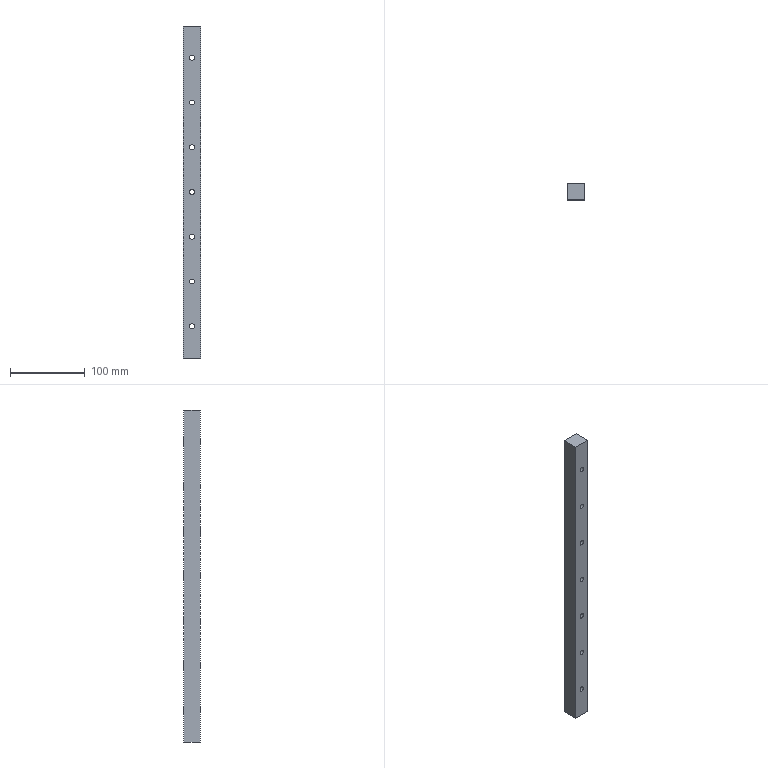Part | SolidWorks | features Extrusion 1, HoleWzd 1, LPattern 1 | 1 solid | 41 faces | box 23 x 22 x 445 mm | volume 217006 mm3 | cylinder 28 | plane 13 | commonest cylinder face diameters 6.6 x14 11 x14
STEP:
#1=CARTESIAN_POINT('',(0.,15.2,37.));
#2=VERTEX_POINT('',#1);
#3=CARTESIAN_POINT('',(0.,15.2,48.));
#4=VERTEX_POINT('',#3);
#5=CARTESIAN_POINT('',(0.,15.2,42.5));
#6=DIRECTION('',(0.,1.,0.));
#7=DIRECTION('',(0.,0.,1.));
#8=AXIS2_PLACEMENT_3D('',#5,#6,#7);
#9=CIRCLE('',#8,5.5);
#10=EDGE_CURVE('',#2,#4,#9,.T.);
#11=ORIENTED_EDGE('',*,*,#10,.F.);
#12=CARTESIAN_POINT('',(0.,22.,37.));
#13=VERTEX_POINT('',#12);
#14=CARTESIAN_POINT('',(0.,22.,37.));
#15=DIRECTION('',(0.,1.,0.));
#16=VECTOR('',#15,1000.);
#17=LINE('',#14,#16);
#18=EDGE_CURVE('',#2,#13,#17,.T.);
#19=ORIENTED_EDGE('',*,*,#18,.T.);
#20=CARTESIAN_POINT('',(0.,22.,48.));
#21=VERTEX_POINT('',#20);
#22=CARTESIAN_POINT('',(0.,22.,42.5));
#23=DIRECTION('',(0.,1.,0.));
#24=DIRECTION('',(0.,0.,1.));
#25=AXIS2_PLACEMENT_3D('',#22,#23,#24);
#26=CIRCLE('',#25,5.5);
#27=EDGE_CURVE('',#13,#21,#26,.T.);
#28=ORIENTED_EDGE('',*,*,#27,.T.);
#29=CARTESIAN_POINT('',(0.,22.,48.));
#30=DIRECTION('',(0.,1.,0.));
#31=VECTOR('',#30,1000.);
#32=LINE('',#29,#31);
#33=EDGE_CURVE('',#4,#21,#32,.T.);
#34=ORIENTED_EDGE('',*,*,#33,.F.);
#35=EDGE_LOOP('',(#11,#19,#28,#34));
#36=FACE_OUTER_BOUND('',#35,.T.);
#37=CARTESIAN_POINT('',(0.,22.,42.5));
#38=DIRECTION('',(0.,1.,0.));
#39=DIRECTION('',(0.,0.,1.));
#40=AXIS2_PLACEMENT_3D('',#37,#38,#39);
#41=CYLINDRICAL_SURFACE('',#40,5.5);
#42=ADVANCED_FACE('',(#36),#41,.F.);
#43=CARTESIAN_POINT('',(0.,0.,39.2));
#44=VERTEX_POINT('',#43);
#45=CARTESIAN_POINT('',(0.,0.,45.8));
#46=VERTEX_POINT('',#45);
#47=CARTESIAN_POINT('',(0.,0.,42.5));
#48=DIRECTION('',(0.,1.,0.));
#49=DIRECTION('',(0.,0.,1.));
#50=AXIS2_PLACEMENT_3D('',#47,#48,#49);
#51=CIRCLE('',#50,3.3);
#52=EDGE_CURVE('',#44,#46,#51,.T.);
#53=ORIENTED_EDGE('',*,*,#52,.F.);
#54=CARTESIAN_POINT('',(0.,15.2,39.2));
#55=VERTEX_POINT('',#54);
#56=CARTESIAN_POINT('',(0.,22.,39.2));
#57=DIRECTION('',(0.,1.,0.));
#58=VECTOR('',#57,1000.);
#59=LINE('',#56,#58);
#60=EDGE_CURVE('',#44,#55,#59,.T.);
#61=ORIENTED_EDGE('',*,*,#60,.T.);
#62=CARTESIAN_POINT('',(0.,15.2,45.8));
#63=VERTEX_POINT('',#62);
#64=CARTESIAN_POINT('',(0.,15.2,42.5));
#65=DIRECTION('',(0.,1.,0.));
#66=DIRECTION('',(0.,0.,1.));
#67=AXIS2_PLACEMENT_3D('',#64,#65,#66);
#68=CIRCLE('',#67,3.3);
#69=EDGE_CURVE('',#55,#63,#68,.T.);
#70=ORIENTED_EDGE('',*,*,#69,.T.);
#71=CARTESIAN_POINT('',(0.,22.,45.8));
#72=DIRECTION('',(0.,1.,0.));
#73=VECTOR('',#72,1000.);
#74=LINE('',#71,#73);
#75=EDGE_CURVE('',#46,#63,#74,.T.);
#76=ORIENTED_EDGE('',*,*,#75,.F.);
#77=EDGE_LOOP('',(#53,#61,#70,#76));
#78=FACE_OUTER_BOUND('',#77,.T.);
#79=CARTESIAN_POINT('',(0.,22.,42.5));
#80=DIRECTION('',(0.,1.,0.));
#81=DIRECTION('',(0.,0.,1.));
#82=AXIS2_PLACEMENT_3D('',#79,#80,#81);
#83=CYLINDRICAL_SURFACE('',#82,3.3);
#84=ADVANCED_FACE('',(#78),#83,.F.);
#85=CARTESIAN_POINT('',(0.,15.2,97.));
#86=VERTEX_POINT('',#85);
#87=CARTESIAN_POINT('',(0.,15.2,108.));
#88=VERTEX_POINT('',#87);
#89=CARTESIAN_POINT('',(0.,15.2,102.5));
#90=DIRECTION('',(0.,1.,0.));
#91=DIRECTION('',(0.,0.,1.));
#92=AXIS2_PLACEMENT_3D('',#89,#90,#91);
#93=CIRCLE('',#92,5.5);
#94=EDGE_CURVE('',#86,#88,#93,.T.);
#95=ORIENTED_EDGE('',*,*,#94,.F.);
#96=CARTESIAN_POINT('',(0.,22.,97.));
#97=VERTEX_POINT('',#96);
#98=CARTESIAN_POINT('',(0.,22.,97.));
#99=DIRECTION('',(0.,1.,0.));
#100=VECTOR('',#99,1000.);
#101=LINE('',#98,#100);
#102=EDGE_CURVE('',#86,#97,#101,.T.);
#103=ORIENTED_EDGE('',*,*,#102,.T.);
#104=CARTESIAN_POINT('',(0.,22.,108.));
#105=VERTEX_POINT('',#104);
#106=CARTESIAN_POINT('',(0.,22.,102.5));
#107=DIRECTION('',(0.,1.,0.));
#108=DIRECTION('',(0.,0.,1.));
#109=AXIS2_PLACEMENT_3D('',#106,#107,#108);
#110=CIRCLE('',#109,5.5);
#111=EDGE_CURVE('',#97,#105,#110,.T.);
#112=ORIENTED_EDGE('',*,*,#111,.T.);
#113=CARTESIAN_POINT('',(0.,22.,108.));
#114=DIRECTION('',(0.,1.,0.));
#115=VECTOR('',#114,1000.);
#116=LINE('',#113,#115);
#117=EDGE_CURVE('',#88,#105,#116,.T.);
#118=ORIENTED_EDGE('',*,*,#117,.F.);
#119=EDGE_LOOP('',(#95,#103,#112,#118));
#120=FACE_OUTER_BOUND('',#119,.T.);
#121=CARTESIAN_POINT('',(0.,22.,102.5));
#122=DIRECTION('',(0.,1.,0.));
#123=DIRECTION('',(0.,0.,1.));
#124=AXIS2_PLACEMENT_3D('',#121,#122,#123);
#125=CYLINDRICAL_SURFACE('',#124,5.5);
#126=ADVANCED_FACE('',(#120),#125,.F.);
#127=CARTESIAN_POINT('',(0.,0.,99.2));
#128=VERTEX_POINT('',#127);
#129=CARTESIAN_POINT('',(0.,0.,105.8));
#130=VERTEX_POINT('',#129);
#131=CARTESIAN_POINT('',(0.,0.,102.5));
#132=DIRECTION('',(0.,1.,0.));
#133=DIRECTION('',(0.,0.,1.));
#134=AXIS2_PLACEMENT_3D('',#131,#132,#133);
#135=CIRCLE('',#134,3.3);
#136=EDGE_CURVE('',#128,#130,#135,.T.);
#137=ORIENTED_EDGE('',*,*,#136,.F.);
#138=CARTESIAN_POINT('',(0.,15.2,99.2));
#139=VERTEX_POINT('',#138);
#140=CARTESIAN_POINT('',(0.,22.,99.2));
#141=DIRECTION('',(0.,1.,0.));
#142=VECTOR('',#141,1000.);
#143=LINE('',#140,#142);
#144=EDGE_CURVE('',#128,#139,#143,.T.);
#145=ORIENTED_EDGE('',*,*,#144,.T.);
#146=CARTESIAN_POINT('',(0.,15.2,105.8));
#147=VERTEX_POINT('',#146);
#148=CARTESIAN_POINT('',(0.,15.2,102.5));
#149=DIRECTION('',(0.,1.,0.));
#150=DIRECTION('',(0.,0.,1.));
#151=AXIS2_PLACEMENT_3D('',#148,#149,#150);
#152=CIRCLE('',#151,3.3);
#153=EDGE_CURVE('',#139,#147,#152,.T.);
#154=ORIENTED_EDGE('',*,*,#153,.T.);
#155=CARTESIAN_POINT('',(0.,22.,105.8));
#156=DIRECTION('',(0.,1.,0.));
#157=VECTOR('',#156,1000.);
#158=LINE('',#155,#157);
#159=EDGE_CURVE('',#130,#147,#158,.T.);
#160=ORIENTED_EDGE('',*,*,#159,.F.);
#161=EDGE_LOOP('',(#137,#145,#154,#160));
#162=FACE_OUTER_BOUND('',#161,.T.);
#163=CARTESIAN_POINT('',(0.,22.,102.5));
#164=DIRECTION('',(0.,1.,0.));
#165=DIRECTION('',(0.,0.,1.));
#166=AXIS2_PLACEMENT_3D('',#163,#164,#165);
#167=CYLINDRICAL_SURFACE('',#166,3.3);
#168=ADVANCED_FACE('',(#162),#167,.F.);
#169=CARTESIAN_POINT('',(0.,15.2,157.));
#170=VERTEX_POINT('',#169);
#171=CARTESIAN_POINT('',(0.,15.2,168.));
#172=VERTEX_POINT('',#171);
#173=CARTESIAN_POINT('',(0.,15.2,162.5));
#174=DIRECTION('',(0.,1.,0.));
#175=DIRECTION('',(0.,0.,1.));
#176=AXIS2_PLACEMENT_3D('',#173,#174,#175);
#177=CIRCLE('',#176,5.5);
#178=EDGE_CURVE('',#170,#172,#177,.T.);
#179=ORIENTED_EDGE('',*,*,#178,.F.);
#180=CARTESIAN_POINT('',(0.,22.,157.));
#181=VERTEX_POINT('',#180);
#182=CARTESIAN_POINT('',(0.,22.,157.));
#183=DIRECTION('',(0.,1.,0.));
#184=VECTOR('',#183,1000.);
#185=LINE('',#182,#184);
#186=EDGE_CURVE('',#170,#181,#185,.T.);
#187=ORIENTED_EDGE('',*,*,#186,.T.);
#188=CARTESIAN_POINT('',(0.,22.,168.));
#189=VERTEX_POINT('',#188);
#190=CARTESIAN_POINT('',(0.,22.,162.5));
#191=DIRECTION('',(0.,1.,0.));
#192=DIRECTION('',(0.,0.,1.));
#193=AXIS2_PLACEMENT_3D('',#190,#191,#192);
#194=CIRCLE('',#193,5.5);
#195=EDGE_CURVE('',#181,#189,#194,.T.);
#196=ORIENTED_EDGE('',*,*,#195,.T.);
#197=CARTESIAN_POINT('',(0.,22.,168.));
#198=DIRECTION('',(0.,1.,0.));
#199=VECTOR('',#198,1000.);
#200=LINE('',#197,#199);
#201=EDGE_CURVE('',#172,#189,#200,.T.);
#202=ORIENTED_EDGE('',*,*,#201,.F.);
#203=EDGE_LOOP('',(#179,#187,#196,#202));
#204=FACE_OUTER_BOUND('',#203,.T.);
#205=CARTESIAN_POINT('',(0.,22.,162.5));
#206=DIRECTION('',(0.,1.,0.));
#207=DIRECTION('',(0.,0.,1.));
#208=AXIS2_PLACEMENT_3D('',#205,#206,#207);
#209=CYLINDRICAL_SURFACE('',#208,5.5);
#210=ADVANCED_FACE('',(#204),#209,.F.);
#211=CARTESIAN_POINT('',(0.,0.,159.2));
#212=VERTEX_POINT('',#211);
#213=CARTESIAN_POINT('',(0.,0.,165.8));
#214=VERTEX_POINT('',#213);
#215=CARTESIAN_POINT('',(0.,0.,162.5));
#216=DIRECTION('',(0.,1.,0.));
#217=DIRECTION('',(0.,0.,1.));
#218=AXIS2_PLACEMENT_3D('',#215,#216,#217);
#219=CIRCLE('',#218,3.3);
#220=EDGE_CURVE('',#212,#214,#219,.T.);
#221=ORIENTED_EDGE('',*,*,#220,.F.);
#222=CARTESIAN_POINT('',(0.,15.2,159.2));
#223=VERTEX_POINT('',#222);
#224=CARTESIAN_POINT('',(0.,22.,159.2));
#225=DIRECTION('',(0.,1.,0.));
#226=VECTOR('',#225,1000.);
#227=LINE('',#224,#226);
#228=EDGE_CURVE('',#212,#223,#227,.T.);
#229=ORIENTED_EDGE('',*,*,#228,.T.);
#230=CARTESIAN_POINT('',(0.,15.2,165.8));
#231=VERTEX_POINT('',#230);
#232=CARTESIAN_POINT('',(0.,15.2,162.5));
#233=DIRECTION('',(0.,1.,0.));
#234=DIRECTION('',(0.,0.,1.));
#235=AXIS2_PLACEMENT_3D('',#232,#233,#234);
#236=CIRCLE('',#235,3.3);
#237=EDGE_CURVE('',#223,#231,#236,.T.);
#238=ORIENTED_EDGE('',*,*,#237,.T.);
#239=CARTESIAN_POINT('',(0.,22.,165.8));
#240=DIRECTION('',(0.,1.,0.));
#241=VECTOR('',#240,1000.);
#242=LINE('',#239,#241);
#243=EDGE_CURVE('',#214,#231,#242,.T.);
#244=ORIENTED_EDGE('',*,*,#243,.F.);
#245=EDGE_LOOP('',(#221,#229,#238,#244));
#246=FACE_OUTER_BOUND('',#245,.T.);
#247=CARTESIAN_POINT('',(0.,22.,162.5));
#248=DIRECTION('',(0.,1.,0.));
#249=DIRECTION('',(0.,0.,1.));
#250=AXIS2_PLACEMENT_3D('',#247,#248,#249);
#251=CYLINDRICAL_SURFACE('',#250,3.3);
#252=ADVANCED_FACE('',(#246),#251,.F.);
#253=CARTESIAN_POINT('',(0.,15.2,217.));
#254=VERTEX_POINT('',#253);
#255=CARTESIAN_POINT('',(0.,15.2,228.));
#256=VERTEX_POINT('',#255);
#257=CARTESIAN_POINT('',(0.,15.2,222.5));
#258=DIRECTION('',(0.,1.,0.));
#259=DIRECTION('',(0.,0.,1.));
#260=AXIS2_PLACEMENT_3D('',#257,#258,#259);
#261=CIRCLE('',#260,5.5);
#262=EDGE_CURVE('',#254,#256,#261,.T.);
#263=ORIENTED_EDGE('',*,*,#262,.F.);
#264=CARTESIAN_POINT('',(0.,22.,217.));
#265=VERTEX_POINT('',#264);
#266=CARTESIAN_POINT('',(0.,22.,217.));
#267=DIRECTION('',(0.,1.,0.));
#268=VECTOR('',#267,1000.);
#269=LINE('',#266,#268);
#270=EDGE_CURVE('',#254,#265,#269,.T.);
#271=ORIENTED_EDGE('',*,*,#270,.T.);
#272=CARTESIAN_POINT('',(0.,22.,228.));
#273=VERTEX_POINT('',#272);
#274=CARTESIAN_POINT('',(0.,22.,222.5));
#275=DIRECTION('',(0.,1.,0.));
#276=DIRECTION('',(0.,0.,1.));
#277=AXIS2_PLACEMENT_3D('',#274,#275,#276);
#278=CIRCLE('',#277,5.5);
#279=EDGE_CURVE('',#265,#273,#278,.T.);
#280=ORIENTED_EDGE('',*,*,#279,.T.);
#281=CARTESIAN_POINT('',(0.,22.,228.));
#282=DIRECTION('',(0.,1.,0.));
#283=VECTOR('',#282,1000.);
#284=LINE('',#281,#283);
#285=EDGE_CURVE('',#256,#273,#284,.T.);
#286=ORIENTED_EDGE('',*,*,#285,.F.);
#287=EDGE_LOOP('',(#263,#271,#280,#286));
#288=FACE_OUTER_BOUND('',#287,.T.);
#289=CARTESIAN_POINT('',(0.,22.,222.5));
#290=DIRECTION('',(0.,1.,0.));
#291=DIRECTION('',(0.,0.,1.));
#292=AXIS2_PLACEMENT_3D('',#289,#290,#291);
#293=CYLINDRICAL_SURFACE('',#292,5.5);
#294=ADVANCED_FACE('',(#288),#293,.F.);
#295=CARTESIAN_POINT('',(0.,0.,219.2));
#296=VERTEX_POINT('',#295);
#297=CARTESIAN_POINT('',(0.,0.,225.8));
#298=VERTEX_POINT('',#297);
#299=CARTESIAN_POINT('',(0.,0.,222.5));
#300=DIRECTION('',(0.,1.,0.));
#301=DIRECTION('',(0.,0.,1.));
#302=AXIS2_PLACEMENT_3D('',#299,#300,#301);
#303=CIRCLE('',#302,3.3);
#304=EDGE_CURVE('',#296,#298,#303,.T.);
#305=ORIENTED_EDGE('',*,*,#304,.F.);
#306=CARTESIAN_POINT('',(0.,15.2,219.2));
#307=VERTEX_POINT('',#306);
#308=CARTESIAN_POINT('',(0.,22.,219.2));
#309=DIRECTION('',(0.,1.,0.));
#310=VECTOR('',#309,1000.);
#311=LINE('',#308,#310);
#312=EDGE_CURVE('',#296,#307,#311,.T.);
#313=ORIENTED_EDGE('',*,*,#312,.T.);
#314=CARTESIAN_POINT('',(0.,15.2,225.8));
#315=VERTEX_POINT('',#314);
#316=CARTESIAN_POINT('',(0.,15.2,222.5));
#317=DIRECTION('',(0.,1.,0.));
#318=DIRECTION('',(0.,0.,1.));
#319=AXIS2_PLACEMENT_3D('',#316,#317,#318);
#320=CIRCLE('',#319,3.3);
#321=EDGE_CURVE('',#307,#315,#320,.T.);
#322=ORIENTED_EDGE('',*,*,#321,.T.);
#323=CARTESIAN_POINT('',(0.,22.,225.8));
#324=DIRECTION('',(0.,1.,0.));
#325=VECTOR('',#324,1000.);
#326=LINE('',#323,#325);
#327=EDGE_CURVE('',#298,#315,#326,.T.);
#328=ORIENTED_EDGE('',*,*,#327,.F.);
#329=EDGE_LOOP('',(#305,#313,#322,#328));
#330=FACE_OUTER_BOUND('',#329,.T.);
#331=CARTESIAN_POINT('',(0.,22.,222.5));
#332=DIRECTION('',(0.,1.,0.));
#333=DIRECTION('',(0.,0.,1.));
#334=AXIS2_PLACEMENT_3D('',#331,#332,#333);
#335=CYLINDRICAL_SURFACE('',#334,3.3);
#336=ADVANCED_FACE('',(#330),#335,.F.);
#337=CARTESIAN_POINT('',(0.,15.2,277.));
#338=VERTEX_POINT('',#337);
#339=CARTESIAN_POINT('',(0.,15.2,288.));
#340=VERTEX_POINT('',#339);
#341=CARTESIAN_POINT('',(0.,15.2,282.5));
#342=DIRECTION('',(0.,1.,0.));
#343=DIRECTION('',(0.,0.,1.));
#344=AXIS2_PLACEMENT_3D('',#341,#342,#343);
#345=CIRCLE('',#344,5.5);
#346=EDGE_CURVE('',#338,#340,#345,.T.);
#347=ORIENTED_EDGE('',*,*,#346,.F.);
#348=CARTESIAN_POINT('',(0.,22.,277.));
#349=VERTEX_POINT('',#348);
#350=CARTESIAN_POINT('',(0.,22.,277.));
#351=DIRECTION('',(0.,1.,0.));
#352=VECTOR('',#351,1000.);
#353=LINE('',#350,#352);
#354=EDGE_CURVE('',#338,#349,#353,.T.);
#355=ORIENTED_EDGE('',*,*,#354,.T.);
#356=CARTESIAN_POINT('',(0.,22.,288.));
#357=VERTEX_POINT('',#356);
#358=CARTESIAN_POINT('',(0.,22.,282.5));
#359=DIRECTION('',(0.,1.,0.));
#360=DIRECTION('',(0.,0.,1.));
#361=AXIS2_PLACEMENT_3D('',#358,#359,#360);
#362=CIRCLE('',#361,5.5);
#363=EDGE_CURVE('',#349,#357,#362,.T.);
#364=ORIENTED_EDGE('',*,*,#363,.T.);
#365=CARTESIAN_POINT('',(0.,22.,288.));
#366=DIRECTION('',(0.,1.,0.));
#367=VECTOR('',#366,1000.);
#368=LINE('',#365,#367);
#369=EDGE_CURVE('',#340,#357,#368,.T.);
#370=ORIENTED_EDGE('',*,*,#369,.F.);
#371=EDGE_LOOP('',(#347,#355,#364,#370));
#372=FACE_OUTER_BOUND('',#371,.T.);
#373=CARTESIAN_POINT('',(0.,22.,282.5));
#374=DIRECTION('',(0.,1.,0.));
#375=DIRECTION('',(0.,0.,1.));
#376=AXIS2_PLACEMENT_3D('',#373,#374,#375);
#377=CYLINDRICAL_SURFACE('',#376,5.5);
#378=ADVANCED_FACE('',(#372),#377,.F.);
#379=CARTESIAN_POINT('',(0.,0.,279.2));
#380=VERTEX_POINT('',#379);
#381=CARTESIAN_POINT('',(0.,0.,285.8));
#382=VERTEX_POINT('',#381);
#383=CARTESIAN_POINT('',(0.,0.,282.5));
#384=DIRECTION('',(0.,1.,0.));
#385=DIRECTION('',(0.,0.,1.));
#386=AXIS2_PLACEMENT_3D('',#383,#384,#385);
#387=CIRCLE('',#386,3.3);
#388=EDGE_CURVE('',#380,#382,#387,.T.);
#389=ORIENTED_EDGE('',*,*,#388,.F.);
#390=CARTESIAN_POINT('',(0.,15.2,279.2));
#391=VERTEX_POINT('',#390);
#392=CARTESIAN_POINT('',(0.,22.,279.2));
#393=DIRECTION('',(0.,1.,0.));
#394=VECTOR('',#393,1000.);
#395=LINE('',#392,#394);
#396=EDGE_CURVE('',#380,#391,#395,.T.);
#397=ORIENTED_EDGE('',*,*,#396,.T.);
#398=CARTESIAN_POINT('',(0.,15.2,285.8));
#399=VERTEX_POINT('',#398);
#400=CARTESIAN_POINT('',(0.,15.2,282.5));
#401=DIRECTION('',(0.,1.,0.));
#402=DIRECTION('',(0.,0.,1.));
#403=AXIS2_PLACEMENT_3D('',#400,#401,#402);
#404=CIRCLE('',#403,3.3);
#405=EDGE_CURVE('',#391,#399,#404,.T.);
#406=ORIENTED_EDGE('',*,*,#405,.T.);
#407=CARTESIAN_POINT('',(0.,22.,285.8));
#408=DIRECTION('',(0.,1.,0.));
#409=VECTOR('',#408,1000.);
#410=LINE('',#407,#409);
#411=EDGE_CURVE('',#382,#399,#410,.T.);
#412=ORIENTED_EDGE('',*,*,#411,.F.);
#413=EDGE_LOOP('',(#389,#397,#406,#412));
#414=FACE_OUTER_BOUND('',#413,.T.);
#415=CARTESIAN_POINT('',(0.,22.,282.5));
#416=DIRECTION('',(0.,1.,0.));
#417=DIRECTION('',(0.,0.,1.));
#418=AXIS2_PLACEMENT_3D('',#415,#416,#417);
#419=CYLINDRICAL_SURFACE('',#418,3.3);
#420=ADVANCED_FACE('',(#414),#419,.F.);
#421=CARTESIAN_POINT('',(0.,15.2,337.));
#422=VERTEX_POINT('',#421);
#423=CARTESIAN_POINT('',(0.,15.2,348.));
#424=VERTEX_POINT('',#423);
#425=CARTESIAN_POINT('',(0.,15.2,342.5));
#426=DIRECTION('',(0.,1.,0.));
#427=DIRECTION('',(0.,0.,1.));
#428=AXIS2_PLACEMENT_3D('',#425,#426,#427);
#429=CIRCLE('',#428,5.5);
#430=EDGE_CURVE('',#422,#424,#429,.T.);
#431=ORIENTED_EDGE('',*,*,#430,.F.);
#432=CARTESIAN_POINT('',(0.,22.,337.));
#433=VERTEX_POINT('',#432);
#434=CARTESIAN_POINT('',(0.,22.,337.));
#435=DIRECTION('',(0.,1.,0.));
#436=VECTOR('',#435,1000.);
#437=LINE('',#434,#436);
#438=EDGE_CURVE('',#422,#433,#437,.T.);
#439=ORIENTED_EDGE('',*,*,#438,.T.);
#440=CARTESIAN_POINT('',(0.,22.,348.));
#441=VERTEX_POINT('',#440);
#442=CARTESIAN_POINT('',(0.,22.,342.5));
#443=DIRECTION('',(0.,1.,0.));
#444=DIRECTION('',(0.,0.,1.));
#445=AXIS2_PLACEMENT_3D('',#442,#443,#444);
#446=CIRCLE('',#445,5.5);
#447=EDGE_CURVE('',#433,#441,#446,.T.);
#448=ORIENTED_EDGE('',*,*,#447,.T.);
#449=CARTESIAN_POINT('',(0.,22.,348.));
#450=DIRECTION('',(0.,1.,0.));
#451=VECTOR('',#450,1000.);
#452=LINE('',#449,#451);
#453=EDGE_CURVE('',#424,#441,#452,.T.);
#454=ORIENTED_EDGE('',*,*,#453,.F.);
#455=EDGE_LOOP('',(#431,#439,#448,#454));
#456=FACE_OUTER_BOUND('',#455,.T.);
#457=CARTESIAN_POINT('',(0.,22.,342.5));
#458=DIRECTION('',(0.,1.,0.));
#459=DIRECTION('',(0.,0.,1.));
#460=AXIS2_PLACEMENT_3D('',#457,#458,#459);
#461=CYLINDRICAL_SURFACE('',#460,5.5);
#462=ADVANCED_FACE('',(#456),#461,.F.);
#463=CARTESIAN_POINT('',(0.,0.,339.2));
#464=VERTEX_POINT('',#463);
#465=CARTESIAN_POINT('',(0.,0.,345.8));
#466=VERTEX_POINT('',#465);
#467=CARTESIAN_POINT('',(0.,0.,342.5));
#468=DIRECTION('',(0.,1.,0.));
#469=DIRECTION('',(0.,0.,1.));
#470=AXIS2_PLACEMENT_3D('',#467,#468,#469);
#471=CIRCLE('',#470,3.3);
#472=EDGE_CURVE('',#464,#466,#471,.T.);
#473=ORIENTED_EDGE('',*,*,#472,.F.);
#474=CARTESIAN_POINT('',(0.,15.2,339.2));
#475=VERTEX_POINT('',#474);
#476=CARTESIAN_POINT('',(0.,22.,339.2));
#477=DIRECTION('',(0.,1.,0.));
#478=VECTOR('',#477,1000.);
#479=LINE('',#476,#478);
#480=EDGE_CURVE('',#464,#475,#479,.T.);
#481=ORIENTED_EDGE('',*,*,#480,.T.);
#482=CARTESIAN_POINT('',(0.,15.2,345.8));
#483=VERTEX_POINT('',#482);
#484=CARTESIAN_POINT('',(0.,15.2,342.5));
#485=DIRECTION('',(0.,1.,0.));
#486=DIRECTION('',(0.,0.,1.));
#487=AXIS2_PLACEMENT_3D('',#484,#485,#486);
#488=CIRCLE('',#487,3.3);
#489=EDGE_CURVE('',#475,#483,#488,.T.);
#490=ORIENTED_EDGE('',*,*,#489,.T.);
#491=CARTESIAN_POINT('',(0.,22.,345.8));
#492=DIRECTION('',(0.,1.,0.));
#493=VECTOR('',#492,1000.);
#494=LINE('',#491,#493);
#495=EDGE_CURVE('',#466,#483,#494,.T.);
#496=ORIENTED_EDGE('',*,*,#495,.F.);
#497=EDGE_LOOP('',(#473,#481,#490,#496));
#498=FACE_OUTER_BOUND('',#497,.T.);
#499=CARTESIAN_POINT('',(0.,22.,342.5));
#500=DIRECTION('',(0.,1.,0.));
#501=DIRECTION('',(0.,0.,1.));
#502=AXIS2_PLACEMENT_3D('',#499,#500,#501);
#503=CYLINDRICAL_SURFACE('',#502,3.3);
#504=ADVANCED_FACE('',(#498),#503,.F.);
#505=CARTESIAN_POINT('',(0.,15.2,397.));
#506=VERTEX_POINT('',#505);
#507=CARTESIAN_POINT('',(0.,15.2,408.));
#508=VERTEX_POINT('',#507);
#509=CARTESIAN_POINT('',(0.,15.2,402.5));
#510=DIRECTION('',(0.,1.,0.));
#511=DIRECTION('',(0.,0.,1.));
#512=AXIS2_PLACEMENT_3D('',#509,#510,#511);
#513=CIRCLE('',#512,5.5);
#514=EDGE_CURVE('',#506,#508,#513,.T.);
#515=ORIENTED_EDGE('',*,*,#514,.F.);
#516=CARTESIAN_POINT('',(0.,22.,397.));
#517=VERTEX_POINT('',#516);
#518=CARTESIAN_POINT('',(0.,22.,397.));
#519=DIRECTION('',(0.,1.,0.));
#520=VECTOR('',#519,1000.);
#521=LINE('',#518,#520);
#522=EDGE_CURVE('',#506,#517,#521,.T.);
#523=ORIENTED_EDGE('',*,*,#522,.T.);
#524=CARTESIAN_POINT('',(0.,22.,408.));
#525=VERTEX_POINT('',#524);
#526=CARTESIAN_POINT('',(0.,22.,402.5));
#527=DIRECTION('',(0.,1.,0.));
#528=DIRECTION('',(0.,0.,1.));
#529=AXIS2_PLACEMENT_3D('',#526,#527,#528);
#530=CIRCLE('',#529,5.5);
#531=EDGE_CURVE('',#517,#525,#530,.T.);
#532=ORIENTED_EDGE('',*,*,#531,.T.);
#533=CARTESIAN_POINT('',(0.,22.,408.));
#534=DIRECTION('',(0.,1.,0.));
#535=VECTOR('',#534,1000.);
#536=LINE('',#533,#535);
#537=EDGE_CURVE('',#508,#525,#536,.T.);
#538=ORIENTED_EDGE('',*,*,#537,.F.);
#539=EDGE_LOOP('',(#515,#523,#532,#538));
#540=FACE_OUTER_BOUND('',#539,.T.);
#541=CARTESIAN_POINT('',(0.,22.,402.5));
#542=DIRECTION('',(0.,1.,0.));
#543=DIRECTION('',(0.,0.,1.));
#544=AXIS2_PLACEMENT_3D('',#541,#542,#543);
#545=CYLINDRICAL_SURFACE('',#544,5.5);
#546=ADVANCED_FACE('',(#540),#545,.F.);
#547=CARTESIAN_POINT('',(0.,0.,399.2));
#548=VERTEX_POINT('',#547);
#549=CARTESIAN_POINT('',(0.,0.,405.8));
#550=VERTEX_POINT('',#549);
#551=CARTESIAN_POINT('',(0.,0.,402.5));
#552=DIRECTION('',(0.,1.,0.));
#553=DIRECTION('',(0.,0.,1.));
#554=AXIS2_PLACEMENT_3D('',#551,#552,#553);
#555=CIRCLE('',#554,3.3);
#556=EDGE_CURVE('',#548,#550,#555,.T.);
#557=ORIENTED_EDGE('',*,*,#556,.F.);
#558=CARTESIAN_POINT('',(0.,15.2,399.2));
#559=VERTEX_POINT('',#558);
#560=CARTESIAN_POINT('',(0.,22.,399.2));
#561=DIRECTION('',(0.,1.,0.));
#562=VECTOR('',#561,1000.);
#563=LINE('',#560,#562);
#564=EDGE_CURVE('',#548,#559,#563,.T.);
#565=ORIENTED_EDGE('',*,*,#564,.T.);
#566=CARTESIAN_POINT('',(0.,15.2,405.8));
#567=VERTEX_POINT('',#566);
#568=CARTESIAN_POINT('',(0.,15.2,402.5));
#569=DIRECTION('',(0.,1.,0.));
#570=DIRECTION('',(0.,0.,1.));
#571=AXIS2_PLACEMENT_3D('',#568,#569,#570);
#572=CIRCLE('',#571,3.3);
#573=EDGE_CURVE('',#559,#567,#572,.T.);
#574=ORIENTED_EDGE('',*,*,#573,.T.);
#575=CARTESIAN_POINT('',(0.,22.,405.8));
#576=DIRECTION('',(0.,1.,0.));
#577=VECTOR('',#576,1000.);
#578=LINE('',#575,#577);
#579=EDGE_CURVE('',#550,#567,#578,.T.);
#580=ORIENTED_EDGE('',*,*,#579,.F.);
#581=EDGE_LOOP('',(#557,#565,#574,#580));
#582=FACE_OUTER_BOUND('',#581,.T.);
#583=CARTESIAN_POINT('',(0.,22.,402.5));
#584=DIRECTION('',(0.,1.,0.));
#585=DIRECTION('',(0.,0.,1.));
#586=AXIS2_PLACEMENT_3D('',#583,#584,#585);
#587=CYLINDRICAL_SURFACE('',#586,3.3);
#588=ADVANCED_FACE('',(#582),#587,.F.);
#589=CARTESIAN_POINT('',(-11.5,22.,0.));
#590=VERTEX_POINT('',#589);
#591=CARTESIAN_POINT('',(-11.5,0.,0.));
#592=VERTEX_POINT('',#591);
#593=CARTESIAN_POINT('',(-11.5,22.,0.));
#594=DIRECTION('',(0.,-1.,0.));
#595=VECTOR('',#594,1000.);
#596=LINE('',#593,#595);
#597=EDGE_CURVE('',#590,#592,#596,.T.);
#598=ORIENTED_EDGE('',*,*,#597,.T.);
#599=CARTESIAN_POINT('',(-11.5,0.,445.));
#600=VERTEX_POINT('',#599);
#601=CARTESIAN_POINT('',(-11.5,0.,445.));
#602=DIRECTION('',(0.,0.,-1.));
#603=VECTOR('',#602,1000.);
#604=LINE('',#601,#603);
#605=EDGE_CURVE('',#600,#592,#604,.T.);
#606=ORIENTED_EDGE('',*,*,#605,.F.);
#607=CARTESIAN_POINT('',(-11.5,22.,445.));
#608=VERTEX_POINT('',#607);
#609=CARTESIAN_POINT('',(-11.5,22.,445.));
#610=DIRECTION('',(0.,-1.,0.));
#611=VECTOR('',#610,1000.);
#612=LINE('',#609,#611);
#613=EDGE_CURVE('',#608,#600,#612,.T.);
#614=ORIENTED_EDGE('',*,*,#613,.F.);
#615=CARTESIAN_POINT('',(-11.5,22.,445.));
#616=DIRECTION('',(0.,0.,-1.));
#617=VECTOR('',#616,1000.);
#618=LINE('',#615,#617);
#619=EDGE_CURVE('',#608,#590,#618,.T.);
#620=ORIENTED_EDGE('',*,*,#619,.T.);
#621=EDGE_LOOP('',(#598,#606,#614,#620));
#622=FACE_OUTER_BOUND('',#621,.T.);
#623=CARTESIAN_POINT('',(-11.5,22.,445.));
#624=DIRECTION('',(1.,0.,0.));
#625=DIRECTION('',(0.,1.,0.));
#626=AXIS2_PLACEMENT_3D('',#623,#624,#625);
#627=PLANE('',#626);
#628=ADVANCED_FACE('',(#622),#627,.F.);
#629=CARTESIAN_POINT('',(0.,0.,42.5));
#630=DIRECTION('',(0.,1.,0.));
#631=DIRECTION('',(0.,0.,1.));
#632=AXIS2_PLACEMENT_3D('',#629,#630,#631);
#633=CIRCLE('',#632,3.3);
#634=EDGE_CURVE('',#46,#44,#633,.T.);
#635=ORIENTED_EDGE('',*,*,#634,.T.);
#636=ORIENTED_EDGE('',*,*,#52,.T.);
#637=EDGE_LOOP('',(#635,#636));
#638=FACE_BOUND('',#637,.T.);
#639=CARTESIAN_POINT('',(0.,0.,102.5));
#640=DIRECTION('',(0.,1.,0.));
#641=DIRECTION('',(0.,0.,1.));
#642=AXIS2_PLACEMENT_3D('',#639,#640,#641);
#643=CIRCLE('',#642,3.3);
#644=EDGE_CURVE('',#130,#128,#643,.T.);
#645=ORIENTED_EDGE('',*,*,#644,.T.);
#646=ORIENTED_EDGE('',*,*,#136,.T.);
#647=EDGE_LOOP('',(#645,#646));
#648=FACE_BOUND('',#647,.T.);
#649=CARTESIAN_POINT('',(0.,0.,162.5));
#650=DIRECTION('',(0.,1.,0.));
#651=DIRECTION('',(0.,0.,1.));
#652=AXIS2_PLACEMENT_3D('',#649,#650,#651);
#653=CIRCLE('',#652,3.3);
#654=EDGE_CURVE('',#214,#212,#653,.T.);
#655=ORIENTED_EDGE('',*,*,#654,.T.);
#656=ORIENTED_EDGE('',*,*,#220,.T.);
#657=EDGE_LOOP('',(#655,#656));
#658=FACE_BOUND('',#657,.T.);
#659=CARTESIAN_POINT('',(0.,0.,222.5));
#660=DIRECTION('',(0.,1.,0.));
#661=DIRECTION('',(0.,0.,1.));
#662=AXIS2_PLACEMENT_3D('',#659,#660,#661);
#663=CIRCLE('',#662,3.3);
#664=EDGE_CURVE('',#298,#296,#663,.T.);
#665=ORIENTED_EDGE('',*,*,#664,.T.);
#666=ORIENTED_EDGE('',*,*,#304,.T.);
#667=EDGE_LOOP('',(#665,#666));
#668=FACE_BOUND('',#667,.T.);
#669=CARTESIAN_POINT('',(0.,0.,282.5));
#670=DIRECTION('',(0.,1.,0.));
#671=DIRECTION('',(0.,0.,1.));
#672=AXIS2_PLACEMENT_3D('',#669,#670,#671);
#673=CIRCLE('',#672,3.3);
#674=EDGE_CURVE('',#382,#380,#673,.T.);
#675=ORIENTED_EDGE('',*,*,#674,.T.);
#676=ORIENTED_EDGE('',*,*,#388,.T.);
#677=EDGE_LOOP('',(#675,#676));
#678=FACE_BOUND('',#677,.T.);
#679=CARTESIAN_POINT('',(0.,0.,342.5));
#680=DIRECTION('',(0.,1.,0.));
#681=DIRECTION('',(0.,0.,1.));
#682=AXIS2_PLACEMENT_3D('',#679,#680,#681);
#683=CIRCLE('',#682,3.3);
#684=EDGE_CURVE('',#466,#464,#683,.T.);
#685=ORIENTED_EDGE('',*,*,#684,.T.);
#686=ORIENTED_EDGE('',*,*,#472,.T.);
#687=EDGE_LOOP('',(#685,#686));
#688=FACE_BOUND('',#687,.T.);
#689=CARTESIAN_POINT('',(0.,0.,402.5));
#690=DIRECTION('',(0.,1.,0.));
#691=DIRECTION('',(0.,0.,1.));
#692=AXIS2_PLACEMENT_3D('',#689,#690,#691);
#693=CIRCLE('',#692,3.3);
#694=EDGE_CURVE('',#550,#548,#693,.T.);
#695=ORIENTED_EDGE('',*,*,#694,.T.);
#696=ORIENTED_EDGE('',*,*,#556,.T.);
#697=EDGE_LOOP('',(#695,#696));
#698=FACE_BOUND('',#697,.T.);
#699=CARTESIAN_POINT('',(11.5,0.,0.));
#700=VERTEX_POINT('',#699);
#701=CARTESIAN_POINT('',(-11.5,0.,0.));
#702=DIRECTION('',(1.,0.,0.));
#703=VECTOR('',#702,1000.);
#704=LINE('',#701,#703);
#705=EDGE_CURVE('',#592,#700,#704,.T.);
#706=ORIENTED_EDGE('',*,*,#705,.T.);
#707=CARTESIAN_POINT('',(11.5,0.,445.));
#708=VERTEX_POINT('',#707);
#709=CARTESIAN_POINT('',(11.5,0.,445.));
#710=DIRECTION('',(0.,0.,-1.));
#711=VECTOR('',#710,1000.);
#712=LINE('',#709,#711);
#713=EDGE_CURVE('',#708,#700,#712,.T.);
#714=ORIENTED_EDGE('',*,*,#713,.F.);
#715=CARTESIAN_POINT('',(-11.5,0.,445.));
#716=DIRECTION('',(1.,0.,0.));
#717=VECTOR('',#716,1000.);
#718=LINE('',#715,#717);
#719=EDGE_CURVE('',#600,#708,#718,.T.);
#720=ORIENTED_EDGE('',*,*,#719,.F.);
#721=ORIENTED_EDGE('',*,*,#605,.T.);
#722=EDGE_LOOP('',(#706,#714,#720,#721));
#723=FACE_OUTER_BOUND('',#722,.T.);
#724=CARTESIAN_POINT('',(-11.5,0.,445.));
#725=DIRECTION('',(0.,1.,0.));
#726=DIRECTION('',(0.,0.,1.));
#727=AXIS2_PLACEMENT_3D('',#724,#725,#726);
#728=PLANE('',#727);
#729=ADVANCED_FACE('',(#638,#648,#658,#668,#678,#688,#698,#723),#728,.F.);
#730=CARTESIAN_POINT('',(11.5,22.,0.));
#731=VERTEX_POINT('',#730);
#732=CARTESIAN_POINT('',(11.5,22.,0.));
#733=DIRECTION('',(0.,1.,0.));
#734=VECTOR('',#733,1000.);
#735=LINE('',#732,#734);
#736=EDGE_CURVE('',#700,#731,#735,.T.);
#737=ORIENTED_EDGE('',*,*,#736,.T.);
#738=CARTESIAN_POINT('',(11.5,22.,445.));
#739=VERTEX_POINT('',#738);
#740=CARTESIAN_POINT('',(11.5,22.,445.));
#741=DIRECTION('',(0.,0.,-1.));
#742=VECTOR('',#741,1000.);
#743=LINE('',#740,#742);
#744=EDGE_CURVE('',#739,#731,#743,.T.);
#745=ORIENTED_EDGE('',*,*,#744,.F.);
#746=CARTESIAN_POINT('',(11.5,22.,445.));
#747=DIRECTION('',(0.,1.,0.));
#748=VECTOR('',#747,1000.);
#749=LINE('',#746,#748);
#750=EDGE_CURVE('',#708,#739,#749,.T.);
#751=ORIENTED_EDGE('',*,*,#750,.F.);
#752=ORIENTED_EDGE('',*,*,#713,.T.);
#753=EDGE_LOOP('',(#737,#745,#751,#752));
#754=FACE_OUTER_BOUND('',#753,.T.);
#755=CARTESIAN_POINT('',(11.5,22.,445.));
#756=DIRECTION('',(-1.,0.,0.));
#757=DIRECTION('',(0.,-1.,0.));
#758=AXIS2_PLACEMENT_3D('',#755,#756,#757);
#759=PLANE('',#758);
#760=ADVANCED_FACE('',(#754),#759,.F.);
#761=CARTESIAN_POINT('',(0.,22.,42.5));
#762=DIRECTION('',(0.,1.,0.));
#763=DIRECTION('',(0.,0.,1.));
#764=AXIS2_PLACEMENT_3D('',#761,#762,#763);
#765=CIRCLE('',#764,5.5);
#766=EDGE_CURVE('',#21,#13,#765,.T.);
#767=ORIENTED_EDGE('',*,*,#766,.F.);
#768=ORIENTED_EDGE('',*,*,#27,.F.);
#769=EDGE_LOOP('',(#767,#768));
#770=FACE_BOUND('',#769,.T.);
#771=CARTESIAN_POINT('',(0.,22.,102.5));
#772=DIRECTION('',(0.,1.,0.));
#773=DIRECTION('',(0.,0.,1.));
#774=AXIS2_PLACEMENT_3D('',#771,#772,#773);
#775=CIRCLE('',#774,5.5);
#776=EDGE_CURVE('',#105,#97,#775,.T.);
#777=ORIENTED_EDGE('',*,*,#776,.F.);
#778=ORIENTED_EDGE('',*,*,#111,.F.);
#779=EDGE_LOOP('',(#777,#778));
#780=FACE_BOUND('',#779,.T.);
#781=CARTESIAN_POINT('',(0.,22.,162.5));
#782=DIRECTION('',(0.,1.,0.));
#783=DIRECTION('',(0.,0.,1.));
#784=AXIS2_PLACEMENT_3D('',#781,#782,#783);
#785=CIRCLE('',#784,5.5);
#786=EDGE_CURVE('',#189,#181,#785,.T.);
#787=ORIENTED_EDGE('',*,*,#786,.F.);
#788=ORIENTED_EDGE('',*,*,#195,.F.);
#789=EDGE_LOOP('',(#787,#788));
#790=FACE_BOUND('',#789,.T.);
#791=CARTESIAN_POINT('',(0.,22.,222.5));
#792=DIRECTION('',(0.,1.,0.));
#793=DIRECTION('',(0.,0.,1.));
#794=AXIS2_PLACEMENT_3D('',#791,#792,#793);
#795=CIRCLE('',#794,5.5);
#796=EDGE_CURVE('',#273,#265,#795,.T.);
#797=ORIENTED_EDGE('',*,*,#796,.F.);
#798=ORIENTED_EDGE('',*,*,#279,.F.);
#799=EDGE_LOOP('',(#797,#798));
#800=FACE_BOUND('',#799,.T.);
#801=CARTESIAN_POINT('',(0.,22.,282.5));
#802=DIRECTION('',(0.,1.,0.));
#803=DIRECTION('',(0.,0.,1.));
#804=AXIS2_PLACEMENT_3D('',#801,#802,#803);
#805=CIRCLE('',#804,5.5);
#806=EDGE_CURVE('',#357,#349,#805,.T.);
#807=ORIENTED_EDGE('',*,*,#806,.F.);
#808=ORIENTED_EDGE('',*,*,#363,.F.);
#809=EDGE_LOOP('',(#807,#808));
#810=FACE_BOUND('',#809,.T.);
#811=CARTESIAN_POINT('',(0.,22.,342.5));
#812=DIRECTION('',(0.,1.,0.));
#813=DIRECTION('',(0.,0.,1.));
#814=AXIS2_PLACEMENT_3D('',#811,#812,#813);
#815=CIRCLE('',#814,5.5);
#816=EDGE_CURVE('',#441,#433,#815,.T.);
#817=ORIENTED_EDGE('',*,*,#816,.F.);
#818=ORIENTED_EDGE('',*,*,#447,.F.);
#819=EDGE_LOOP('',(#817,#818));
#820=FACE_BOUND('',#819,.T.);
#821=CARTESIAN_POINT('',(0.,22.,402.5));
#822=DIRECTION('',(0.,1.,0.));
#823=DIRECTION('',(0.,0.,1.));
#824=AXIS2_PLACEMENT_3D('',#821,#822,#823);
#825=CIRCLE('',#824,5.5);
#826=EDGE_CURVE('',#525,#517,#825,.T.);
#827=ORIENTED_EDGE('',*,*,#826,.F.);
#828=ORIENTED_EDGE('',*,*,#531,.F.);
#829=EDGE_LOOP('',(#827,#828));
#830=FACE_BOUND('',#829,.T.);
#831=CARTESIAN_POINT('',(-11.5,22.,0.));
#832=DIRECTION('',(-1.,0.,0.));
#833=VECTOR('',#832,1000.);
#834=LINE('',#831,#833);
#835=EDGE_CURVE('',#731,#590,#834,.T.);
#836=ORIENTED_EDGE('',*,*,#835,.T.);
#837=ORIENTED_EDGE('',*,*,#619,.F.);
#838=CARTESIAN_POINT('',(-11.5,22.,445.));
#839=DIRECTION('',(-1.,0.,0.));
#840=VECTOR('',#839,1000.);
#841=LINE('',#838,#840);
#842=EDGE_CURVE('',#739,#608,#841,.T.);
#843=ORIENTED_EDGE('',*,*,#842,.F.);
#844=ORIENTED_EDGE('',*,*,#744,.T.);
#845=EDGE_LOOP('',(#836,#837,#843,#844));
#846=FACE_OUTER_BOUND('',#845,.T.);
#847=CARTESIAN_POINT('',(-11.5,22.,445.));
#848=DIRECTION('',(0.,-1.,0.));
#849=DIRECTION('',(0.,0.,-1.));
#850=AXIS2_PLACEMENT_3D('',#847,#848,#849);
#851=PLANE('',#850);
#852=ADVANCED_FACE('',(#770,#780,#790,#800,#810,#820,#830,#846),#851,.F.);
#853=ORIENTED_EDGE('',*,*,#613,.T.);
#854=ORIENTED_EDGE('',*,*,#719,.T.);
#855=ORIENTED_EDGE('',*,*,#750,.T.);
#856=ORIENTED_EDGE('',*,*,#842,.T.);
#857=EDGE_LOOP('',(#853,#854,#855,#856));
#858=FACE_OUTER_BOUND('',#857,.T.);
#859=CARTESIAN_POINT('',(0.,0.,445.));
#860=DIRECTION('',(0.,0.,1.));
#861=DIRECTION('',(1.,0.,0.));
#862=AXIS2_PLACEMENT_3D('',#859,#860,#861);
#863=PLANE('',#862);
#864=ADVANCED_FACE('',(#858),#863,.T.);
#865=ORIENTED_EDGE('',*,*,#597,.F.);
#866=ORIENTED_EDGE('',*,*,#835,.F.);
#867=ORIENTED_EDGE('',*,*,#736,.F.);
#868=ORIENTED_EDGE('',*,*,#705,.F.);
#869=EDGE_LOOP('',(#865,#866,#867,#868));
#870=FACE_OUTER_BOUND('',#869,.T.);
#871=CARTESIAN_POINT('',(0.,0.,0.));
#872=DIRECTION('',(0.,0.,1.));
#873=DIRECTION('',(1.,0.,0.));
#874=AXIS2_PLACEMENT_3D('',#871,#872,#873);
#875=PLANE('',#874);
#876=ADVANCED_FACE('',(#870),#875,.F.);
#877=ORIENTED_EDGE('',*,*,#564,.F.);
#878=ORIENTED_EDGE('',*,*,#694,.F.);
#879=ORIENTED_EDGE('',*,*,#579,.T.);
#880=CARTESIAN_POINT('',(0.,15.2,402.5));
#881=DIRECTION('',(0.,1.,0.));
#882=DIRECTION('',(0.,0.,1.));
#883=AXIS2_PLACEMENT_3D('',#880,#881,#882);
#884=CIRCLE('',#883,3.3);
#885=EDGE_CURVE('',#567,#559,#884,.T.);
#886=ORIENTED_EDGE('',*,*,#885,.T.);
#887=EDGE_LOOP('',(#877,#878,#879,#886));
#888=FACE_OUTER_BOUND('',#887,.T.);
#889=CARTESIAN_POINT('',(0.,22.,402.5));
#890=DIRECTION('',(0.,1.,0.));
#891=DIRECTION('',(0.,0.,1.));
#892=AXIS2_PLACEMENT_3D('',#889,#890,#891);
#893=CYLINDRICAL_SURFACE('',#892,3.3);
#894=ADVANCED_FACE('',(#888),#893,.F.);
#895=ORIENTED_EDGE('',*,*,#885,.F.);
#896=ORIENTED_EDGE('',*,*,#573,.F.);
#897=EDGE_LOOP('',(#895,#896));
#898=FACE_BOUND('',#897,.T.);
#899=CARTESIAN_POINT('',(0.,15.2,402.5));
#900=DIRECTION('',(0.,1.,0.));
#901=DIRECTION('',(0.,0.,1.));
#902=AXIS2_PLACEMENT_3D('',#899,#900,#901);
#903=CIRCLE('',#902,5.5);
#904=EDGE_CURVE('',#508,#506,#903,.T.);
#905=ORIENTED_EDGE('',*,*,#904,.T.);
#906=ORIENTED_EDGE('',*,*,#514,.T.);
#907=EDGE_LOOP('',(#905,#906));
#908=FACE_OUTER_BOUND('',#907,.T.);
#909=CARTESIAN_POINT('',(3.3,15.2,402.5));
#910=DIRECTION('',(0.,-1.,0.));
#911=DIRECTION('',(0.,0.,-1.));
#912=AXIS2_PLACEMENT_3D('',#909,#910,#911);
#913=PLANE('',#912);
#914=ADVANCED_FACE('',(#898,#908),#913,.F.);
#915=ORIENTED_EDGE('',*,*,#522,.F.);
#916=ORIENTED_EDGE('',*,*,#904,.F.);
#917=ORIENTED_EDGE('',*,*,#537,.T.);
#918=ORIENTED_EDGE('',*,*,#826,.T.);
#919=EDGE_LOOP('',(#915,#916,#917,#918));
#920=FACE_OUTER_BOUND('',#919,.T.);
#921=CARTESIAN_POINT('',(0.,22.,402.5));
#922=DIRECTION('',(0.,1.,0.));
#923=DIRECTION('',(0.,0.,1.));
#924=AXIS2_PLACEMENT_3D('',#921,#922,#923);
#925=CYLINDRICAL_SURFACE('',#924,5.5);
#926=ADVANCED_FACE('',(#920),#925,.F.);
#927=ORIENTED_EDGE('',*,*,#480,.F.);
#928=ORIENTED_EDGE('',*,*,#684,.F.);
#929=ORIENTED_EDGE('',*,*,#495,.T.);
#930=CARTESIAN_POINT('',(0.,15.2,342.5));
#931=DIRECTION('',(0.,1.,0.));
#932=DIRECTION('',(0.,0.,1.));
#933=AXIS2_PLACEMENT_3D('',#930,#931,#932);
#934=CIRCLE('',#933,3.3);
#935=EDGE_CURVE('',#483,#475,#934,.T.);
#936=ORIENTED_EDGE('',*,*,#935,.T.);
#937=EDGE_LOOP('',(#927,#928,#929,#936));
#938=FACE_OUTER_BOUND('',#937,.T.);
#939=CARTESIAN_POINT('',(0.,22.,342.5));
#940=DIRECTION('',(0.,1.,0.));
#941=DIRECTION('',(0.,0.,1.));
#942=AXIS2_PLACEMENT_3D('',#939,#940,#941);
#943=CYLINDRICAL_SURFACE('',#942,3.3);
#944=ADVANCED_FACE('',(#938),#943,.F.);
#945=ORIENTED_EDGE('',*,*,#935,.F.);
#946=ORIENTED_EDGE('',*,*,#489,.F.);
#947=EDGE_LOOP('',(#945,#946));
#948=FACE_BOUND('',#947,.T.);
#949=CARTESIAN_POINT('',(0.,15.2,342.5));
#950=DIRECTION('',(0.,1.,0.));
#951=DIRECTION('',(0.,0.,1.));
#952=AXIS2_PLACEMENT_3D('',#949,#950,#951);
#953=CIRCLE('',#952,5.5);
#954=EDGE_CURVE('',#424,#422,#953,.T.);
#955=ORIENTED_EDGE('',*,*,#954,.T.);
#956=ORIENTED_EDGE('',*,*,#430,.T.);
#957=EDGE_LOOP('',(#955,#956));
#958=FACE_OUTER_BOUND('',#957,.T.);
#959=CARTESIAN_POINT('',(3.3,15.2,342.5));
#960=DIRECTION('',(0.,-1.,0.));
#961=DIRECTION('',(0.,0.,-1.));
#962=AXIS2_PLACEMENT_3D('',#959,#960,#961);
#963=PLANE('',#962);
#964=ADVANCED_FACE('',(#948,#958),#963,.F.);
#965=ORIENTED_EDGE('',*,*,#438,.F.);
#966=ORIENTED_EDGE('',*,*,#954,.F.);
#967=ORIENTED_EDGE('',*,*,#453,.T.);
#968=ORIENTED_EDGE('',*,*,#816,.T.);
#969=EDGE_LOOP('',(#965,#966,#967,#968));
#970=FACE_OUTER_BOUND('',#969,.T.);
#971=CARTESIAN_POINT('',(0.,22.,342.5));
#972=DIRECTION('',(0.,1.,0.));
#973=DIRECTION('',(0.,0.,1.));
#974=AXIS2_PLACEMENT_3D('',#971,#972,#973);
#975=CYLINDRICAL_SURFACE('',#974,5.5);
#976=ADVANCED_FACE('',(#970),#975,.F.);
#977=ORIENTED_EDGE('',*,*,#396,.F.);
#978=ORIENTED_EDGE('',*,*,#674,.F.);
#979=ORIENTED_EDGE('',*,*,#411,.T.);
#980=CARTESIAN_POINT('',(0.,15.2,282.5));
#981=DIRECTION('',(0.,1.,0.));
#982=DIRECTION('',(0.,0.,1.));
#983=AXIS2_PLACEMENT_3D('',#980,#981,#982);
#984=CIRCLE('',#983,3.3);
#985=EDGE_CURVE('',#399,#391,#984,.T.);
#986=ORIENTED_EDGE('',*,*,#985,.T.);
#987=EDGE_LOOP('',(#977,#978,#979,#986));
#988=FACE_OUTER_BOUND('',#987,.T.);
#989=CARTESIAN_POINT('',(0.,22.,282.5));
#990=DIRECTION('',(0.,1.,0.));
#991=DIRECTION('',(0.,0.,1.));
#992=AXIS2_PLACEMENT_3D('',#989,#990,#991);
#993=CYLINDRICAL_SURFACE('',#992,3.3);
#994=ADVANCED_FACE('',(#988),#993,.F.);
#995=ORIENTED_EDGE('',*,*,#985,.F.);
#996=ORIENTED_EDGE('',*,*,#405,.F.);
#997=EDGE_LOOP('',(#995,#996));
#998=FACE_BOUND('',#997,.T.);
#999=CARTESIAN_POINT('',(0.,15.2,282.5));
#1000=DIRECTION('',(0.,1.,0.));
#1001=DIRECTION('',(0.,0.,1.));
#1002=AXIS2_PLACEMENT_3D('',#999,#1000,#1001);
#1003=CIRCLE('',#1002,5.5);
#1004=EDGE_CURVE('',#340,#338,#1003,.T.);
#1005=ORIENTED_EDGE('',*,*,#1004,.T.);
#1006=ORIENTED_EDGE('',*,*,#346,.T.);
#1007=EDGE_LOOP('',(#1005,#1006));
#1008=FACE_OUTER_BOUND('',#1007,.T.);
#1009=CARTESIAN_POINT('',(3.3,15.2,282.5));
#1010=DIRECTION('',(0.,-1.,0.));
#1011=DIRECTION('',(0.,0.,-1.));
#1012=AXIS2_PLACEMENT_3D('',#1009,#1010,#1011);
#1013=PLANE('',#1012);
#1014=ADVANCED_FACE('',(#998,#1008),#1013,.F.);
#1015=ORIENTED_EDGE('',*,*,#354,.F.);
#1016=ORIENTED_EDGE('',*,*,#1004,.F.);
#1017=ORIENTED_EDGE('',*,*,#369,.T.);
#1018=ORIENTED_EDGE('',*,*,#806,.T.);
#1019=EDGE_LOOP('',(#1015,#1016,#1017,#1018));
#1020=FACE_OUTER_BOUND('',#1019,.T.);
#1021=CARTESIAN_POINT('',(0.,22.,282.5));
#1022=DIRECTION('',(0.,1.,0.));
#1023=DIRECTION('',(0.,0.,1.));
#1024=AXIS2_PLACEMENT_3D('',#1021,#1022,#1023);
#1025=CYLINDRICAL_SURFACE('',#1024,5.5);
#1026=ADVANCED_FACE('',(#1020),#1025,.F.);
#1027=ORIENTED_EDGE('',*,*,#312,.F.);
#1028=ORIENTED_EDGE('',*,*,#664,.F.);
#1029=ORIENTED_EDGE('',*,*,#327,.T.);
#1030=CARTESIAN_POINT('',(0.,15.2,222.5));
#1031=DIRECTION('',(0.,1.,0.));
#1032=DIRECTION('',(0.,0.,1.));
#1033=AXIS2_PLACEMENT_3D('',#1030,#1031,#1032);
#1034=CIRCLE('',#1033,3.3);
#1035=EDGE_CURVE('',#315,#307,#1034,.T.);
#1036=ORIENTED_EDGE('',*,*,#1035,.T.);
#1037=EDGE_LOOP('',(#1027,#1028,#1029,#1036));
#1038=FACE_OUTER_BOUND('',#1037,.T.);
#1039=CARTESIAN_POINT('',(0.,22.,222.5));
#1040=DIRECTION('',(0.,1.,0.));
#1041=DIRECTION('',(0.,0.,1.));
#1042=AXIS2_PLACEMENT_3D('',#1039,#1040,#1041);
#1043=CYLINDRICAL_SURFACE('',#1042,3.3);
#1044=ADVANCED_FACE('',(#1038),#1043,.F.);
#1045=ORIENTED_EDGE('',*,*,#1035,.F.);
#1046=ORIENTED_EDGE('',*,*,#321,.F.);
#1047=EDGE_LOOP('',(#1045,#1046));
#1048=FACE_BOUND('',#1047,.T.);
#1049=CARTESIAN_POINT('',(0.,15.2,222.5));
#1050=DIRECTION('',(0.,1.,0.));
#1051=DIRECTION('',(0.,0.,1.));
#1052=AXIS2_PLACEMENT_3D('',#1049,#1050,#1051);
#1053=CIRCLE('',#1052,5.5);
#1054=EDGE_CURVE('',#256,#254,#1053,.T.);
#1055=ORIENTED_EDGE('',*,*,#1054,.T.);
#1056=ORIENTED_EDGE('',*,*,#262,.T.);
#1057=EDGE_LOOP('',(#1055,#1056));
#1058=FACE_OUTER_BOUND('',#1057,.T.);
#1059=CARTESIAN_POINT('',(3.3,15.2,222.5));
#1060=DIRECTION('',(0.,-1.,0.));
#1061=DIRECTION('',(0.,0.,-1.));
#1062=AXIS2_PLACEMENT_3D('',#1059,#1060,#1061);
#1063=PLANE('',#1062);
#1064=ADVANCED_FACE('',(#1048,#1058),#1063,.F.);
#1065=ORIENTED_EDGE('',*,*,#270,.F.);
#1066=ORIENTED_EDGE('',*,*,#1054,.F.);
#1067=ORIENTED_EDGE('',*,*,#285,.T.);
#1068=ORIENTED_EDGE('',*,*,#796,.T.);
#1069=EDGE_LOOP('',(#1065,#1066,#1067,#1068));
#1070=FACE_OUTER_BOUND('',#1069,.T.);
#1071=CARTESIAN_POINT('',(0.,22.,222.5));
#1072=DIRECTION('',(0.,1.,0.));
#1073=DIRECTION('',(0.,0.,1.));
#1074=AXIS2_PLACEMENT_3D('',#1071,#1072,#1073);
#1075=CYLINDRICAL_SURFACE('',#1074,5.5);
#1076=ADVANCED_FACE('',(#1070),#1075,.F.);
#1077=ORIENTED_EDGE('',*,*,#228,.F.);
#1078=ORIENTED_EDGE('',*,*,#654,.F.);
#1079=ORIENTED_EDGE('',*,*,#243,.T.);
#1080=CARTESIAN_POINT('',(0.,15.2,162.5));
#1081=DIRECTION('',(0.,1.,0.));
#1082=DIRECTION('',(0.,0.,1.));
#1083=AXIS2_PLACEMENT_3D('',#1080,#1081,#1082);
#1084=CIRCLE('',#1083,3.3);
#1085=EDGE_CURVE('',#231,#223,#1084,.T.);
#1086=ORIENTED_EDGE('',*,*,#1085,.T.);
#1087=EDGE_LOOP('',(#1077,#1078,#1079,#1086));
#1088=FACE_OUTER_BOUND('',#1087,.T.);
#1089=CARTESIAN_POINT('',(0.,22.,162.5));
#1090=DIRECTION('',(0.,1.,0.));
#1091=DIRECTION('',(0.,0.,1.));
#1092=AXIS2_PLACEMENT_3D('',#1089,#1090,#1091);
#1093=CYLINDRICAL_SURFACE('',#1092,3.3);
#1094=ADVANCED_FACE('',(#1088),#1093,.F.);
#1095=ORIENTED_EDGE('',*,*,#1085,.F.);
#1096=ORIENTED_EDGE('',*,*,#237,.F.);
#1097=EDGE_LOOP('',(#1095,#1096));
#1098=FACE_BOUND('',#1097,.T.);
#1099=CARTESIAN_POINT('',(0.,15.2,162.5));
#1100=DIRECTION('',(0.,1.,0.));
#1101=DIRECTION('',(0.,0.,1.));
#1102=AXIS2_PLACEMENT_3D('',#1099,#1100,#1101);
#1103=CIRCLE('',#1102,5.5);
#1104=EDGE_CURVE('',#172,#170,#1103,.T.);
#1105=ORIENTED_EDGE('',*,*,#1104,.T.);
#1106=ORIENTED_EDGE('',*,*,#178,.T.);
#1107=EDGE_LOOP('',(#1105,#1106));
#1108=FACE_OUTER_BOUND('',#1107,.T.);
#1109=CARTESIAN_POINT('',(3.3,15.2,162.5));
#1110=DIRECTION('',(0.,-1.,0.));
#1111=DIRECTION('',(0.,0.,-1.));
#1112=AXIS2_PLACEMENT_3D('',#1109,#1110,#1111);
#1113=PLANE('',#1112);
#1114=ADVANCED_FACE('',(#1098,#1108),#1113,.F.);
#1115=ORIENTED_EDGE('',*,*,#186,.F.);
#1116=ORIENTED_EDGE('',*,*,#1104,.F.);
#1117=ORIENTED_EDGE('',*,*,#201,.T.);
#1118=ORIENTED_EDGE('',*,*,#786,.T.);
#1119=EDGE_LOOP('',(#1115,#1116,#1117,#1118));
#1120=FACE_OUTER_BOUND('',#1119,.T.);
#1121=CARTESIAN_POINT('',(0.,22.,162.5));
#1122=DIRECTION('',(0.,1.,0.));
#1123=DIRECTION('',(0.,0.,1.));
#1124=AXIS2_PLACEMENT_3D('',#1121,#1122,#1123);
#1125=CYLINDRICAL_SURFACE('',#1124,5.5);
#1126=ADVANCED_FACE('',(#1120),#1125,.F.);
#1127=ORIENTED_EDGE('',*,*,#144,.F.);
#1128=ORIENTED_EDGE('',*,*,#644,.F.);
#1129=ORIENTED_EDGE('',*,*,#159,.T.);
#1130=CARTESIAN_POINT('',(0.,15.2,102.5));
#1131=DIRECTION('',(0.,1.,0.));
#1132=DIRECTION('',(0.,0.,1.));
#1133=AXIS2_PLACEMENT_3D('',#1130,#1131,#1132);
#1134=CIRCLE('',#1133,3.3);
#1135=EDGE_CURVE('',#147,#139,#1134,.T.);
#1136=ORIENTED_EDGE('',*,*,#1135,.T.);
#1137=EDGE_LOOP('',(#1127,#1128,#1129,#1136));
#1138=FACE_OUTER_BOUND('',#1137,.T.);
#1139=CARTESIAN_POINT('',(0.,22.,102.5));
#1140=DIRECTION('',(0.,1.,0.));
#1141=DIRECTION('',(0.,0.,1.));
#1142=AXIS2_PLACEMENT_3D('',#1139,#1140,#1141);
#1143=CYLINDRICAL_SURFACE('',#1142,3.3);
#1144=ADVANCED_FACE('',(#1138),#1143,.F.);
#1145=ORIENTED_EDGE('',*,*,#1135,.F.);
#1146=ORIENTED_EDGE('',*,*,#153,.F.);
#1147=EDGE_LOOP('',(#1145,#1146));
#1148=FACE_BOUND('',#1147,.T.);
#1149=CARTESIAN_POINT('',(0.,15.2,102.5));
#1150=DIRECTION('',(0.,1.,0.));
#1151=DIRECTION('',(0.,0.,1.));
#1152=AXIS2_PLACEMENT_3D('',#1149,#1150,#1151);
#1153=CIRCLE('',#1152,5.5);
#1154=EDGE_CURVE('',#88,#86,#1153,.T.);
#1155=ORIENTED_EDGE('',*,*,#1154,.T.);
#1156=ORIENTED_EDGE('',*,*,#94,.T.);
#1157=EDGE_LOOP('',(#1155,#1156));
#1158=FACE_OUTER_BOUND('',#1157,.T.);
#1159=CARTESIAN_POINT('',(3.3,15.2,102.5));
#1160=DIRECTION('',(0.,-1.,0.));
#1161=DIRECTION('',(0.,0.,-1.));
#1162=AXIS2_PLACEMENT_3D('',#1159,#1160,#1161);
#1163=PLANE('',#1162);
#1164=ADVANCED_FACE('',(#1148,#1158),#1163,.F.);
#1165=ORIENTED_EDGE('',*,*,#102,.F.);
#1166=ORIENTED_EDGE('',*,*,#1154,.F.);
#1167=ORIENTED_EDGE('',*,*,#117,.T.);
#1168=ORIENTED_EDGE('',*,*,#776,.T.);
#1169=EDGE_LOOP('',(#1165,#1166,#1167,#1168));
#1170=FACE_OUTER_BOUND('',#1169,.T.);
#1171=CARTESIAN_POINT('',(0.,22.,102.5));
#1172=DIRECTION('',(0.,1.,0.));
#1173=DIRECTION('',(0.,0.,1.));
#1174=AXIS2_PLACEMENT_3D('',#1171,#1172,#1173);
#1175=CYLINDRICAL_SURFACE('',#1174,5.5);
#1176=ADVANCED_FACE('',(#1170),#1175,.F.);
#1177=ORIENTED_EDGE('',*,*,#60,.F.);
#1178=ORIENTED_EDGE('',*,*,#634,.F.);
#1179=ORIENTED_EDGE('',*,*,#75,.T.);
#1180=CARTESIAN_POINT('',(0.,15.2,42.5));
#1181=DIRECTION('',(0.,1.,0.));
#1182=DIRECTION('',(0.,0.,1.));
#1183=AXIS2_PLACEMENT_3D('',#1180,#1181,#1182);
#1184=CIRCLE('',#1183,3.3);
#1185=EDGE_CURVE('',#63,#55,#1184,.T.);
#1186=ORIENTED_EDGE('',*,*,#1185,.T.);
#1187=EDGE_LOOP('',(#1177,#1178,#1179,#1186));
#1188=FACE_OUTER_BOUND('',#1187,.T.);
#1189=CARTESIAN_POINT('',(0.,22.,42.5));
#1190=DIRECTION('',(0.,1.,0.));
#1191=DIRECTION('',(0.,0.,1.));
#1192=AXIS2_PLACEMENT_3D('',#1189,#1190,#1191);
#1193=CYLINDRICAL_SURFACE('',#1192,3.3);
#1194=ADVANCED_FACE('',(#1188),#1193,.F.);
#1195=ORIENTED_EDGE('',*,*,#1185,.F.);
#1196=ORIENTED_EDGE('',*,*,#69,.F.);
#1197=EDGE_LOOP('',(#1195,#1196));
#1198=FACE_BOUND('',#1197,.T.);
#1199=CARTESIAN_POINT('',(0.,15.2,42.5));
#1200=DIRECTION('',(0.,1.,0.));
#1201=DIRECTION('',(0.,0.,1.));
#1202=AXIS2_PLACEMENT_3D('',#1199,#1200,#1201);
#1203=CIRCLE('',#1202,5.5);
#1204=EDGE_CURVE('',#4,#2,#1203,.T.);
#1205=ORIENTED_EDGE('',*,*,#1204,.T.);
#1206=ORIENTED_EDGE('',*,*,#10,.T.);
#1207=EDGE_LOOP('',(#1205,#1206));
#1208=FACE_OUTER_BOUND('',#1207,.T.);
#1209=CARTESIAN_POINT('',(3.3,15.2,42.5));
#1210=DIRECTION('',(0.,-1.,0.));
#1211=DIRECTION('',(0.,0.,-1.));
#1212=AXIS2_PLACEMENT_3D('',#1209,#1210,#1211);
#1213=PLANE('',#1212);
#1214=ADVANCED_FACE('',(#1198,#1208),#1213,.F.);
#1215=ORIENTED_EDGE('',*,*,#18,.F.);
#1216=ORIENTED_EDGE('',*,*,#1204,.F.);
#1217=ORIENTED_EDGE('',*,*,#33,.T.);
#1218=ORIENTED_EDGE('',*,*,#766,.T.);
#1219=EDGE_LOOP('',(#1215,#1216,#1217,#1218));
#1220=FACE_OUTER_BOUND('',#1219,.T.);
#1221=CARTESIAN_POINT('',(0.,22.,42.5));
#1222=DIRECTION('',(0.,1.,0.));
#1223=DIRECTION('',(0.,0.,1.));
#1224=AXIS2_PLACEMENT_3D('',#1221,#1222,#1223);
#1225=CYLINDRICAL_SURFACE('',#1224,5.5);
#1226=ADVANCED_FACE('',(#1220),#1225,.F.);
#1227=CLOSED_SHELL('',(#42,#84,#126,#168,#210,#252,#294,#336,#378,#420,#462,#504,#546,#588,#628,#729,#760,#852,#864,#876,#894,#914,#926,#944,#964,#976,#994,#1014,#1026,#1044,#1064,#1076,#1094,#1114,#1126,#1144,#1164,#1176,#1194,#1214,#1226));
#1228=MANIFOLD_SOLID_BREP('',#1227);
#1229=CARTESIAN_POINT('',(0.,0.,0.));
#1230=DIRECTION('',(0.,0.,1.));
#1231=DIRECTION('',(1.,0.,0.));
#1232=AXIS2_PLACEMENT_3D('',#1229,#1230,#1231);
#1233=(LENGTH_UNIT()NAMED_UNIT(*)SI_UNIT(.MILLI.,.METRE.));
#1234=UNCERTAINTY_MEASURE_WITH_UNIT(LENGTH_MEASURE(0.00001),#1233,'','');
#1235=(NAMED_UNIT(*)PLANE_ANGLE_UNIT()SI_UNIT($,.RADIAN.));
#1236=(NAMED_UNIT(*)SI_UNIT($,.STERADIAN.)SOLID_ANGLE_UNIT());
#1237=(GEOMETRIC_REPRESENTATION_CONTEXT(3)GLOBAL_UNCERTAINTY_ASSIGNED_CONTEXT((#1234))GLOBAL_UNIT_ASSIGNED_CONTEXT((#1233,#1235,#1236))REPRESENTATION_CONTEXT('',''));
#1238=ADVANCED_BREP_SHAPE_REPRESENTATION('',(#1228,#1232),#1237);